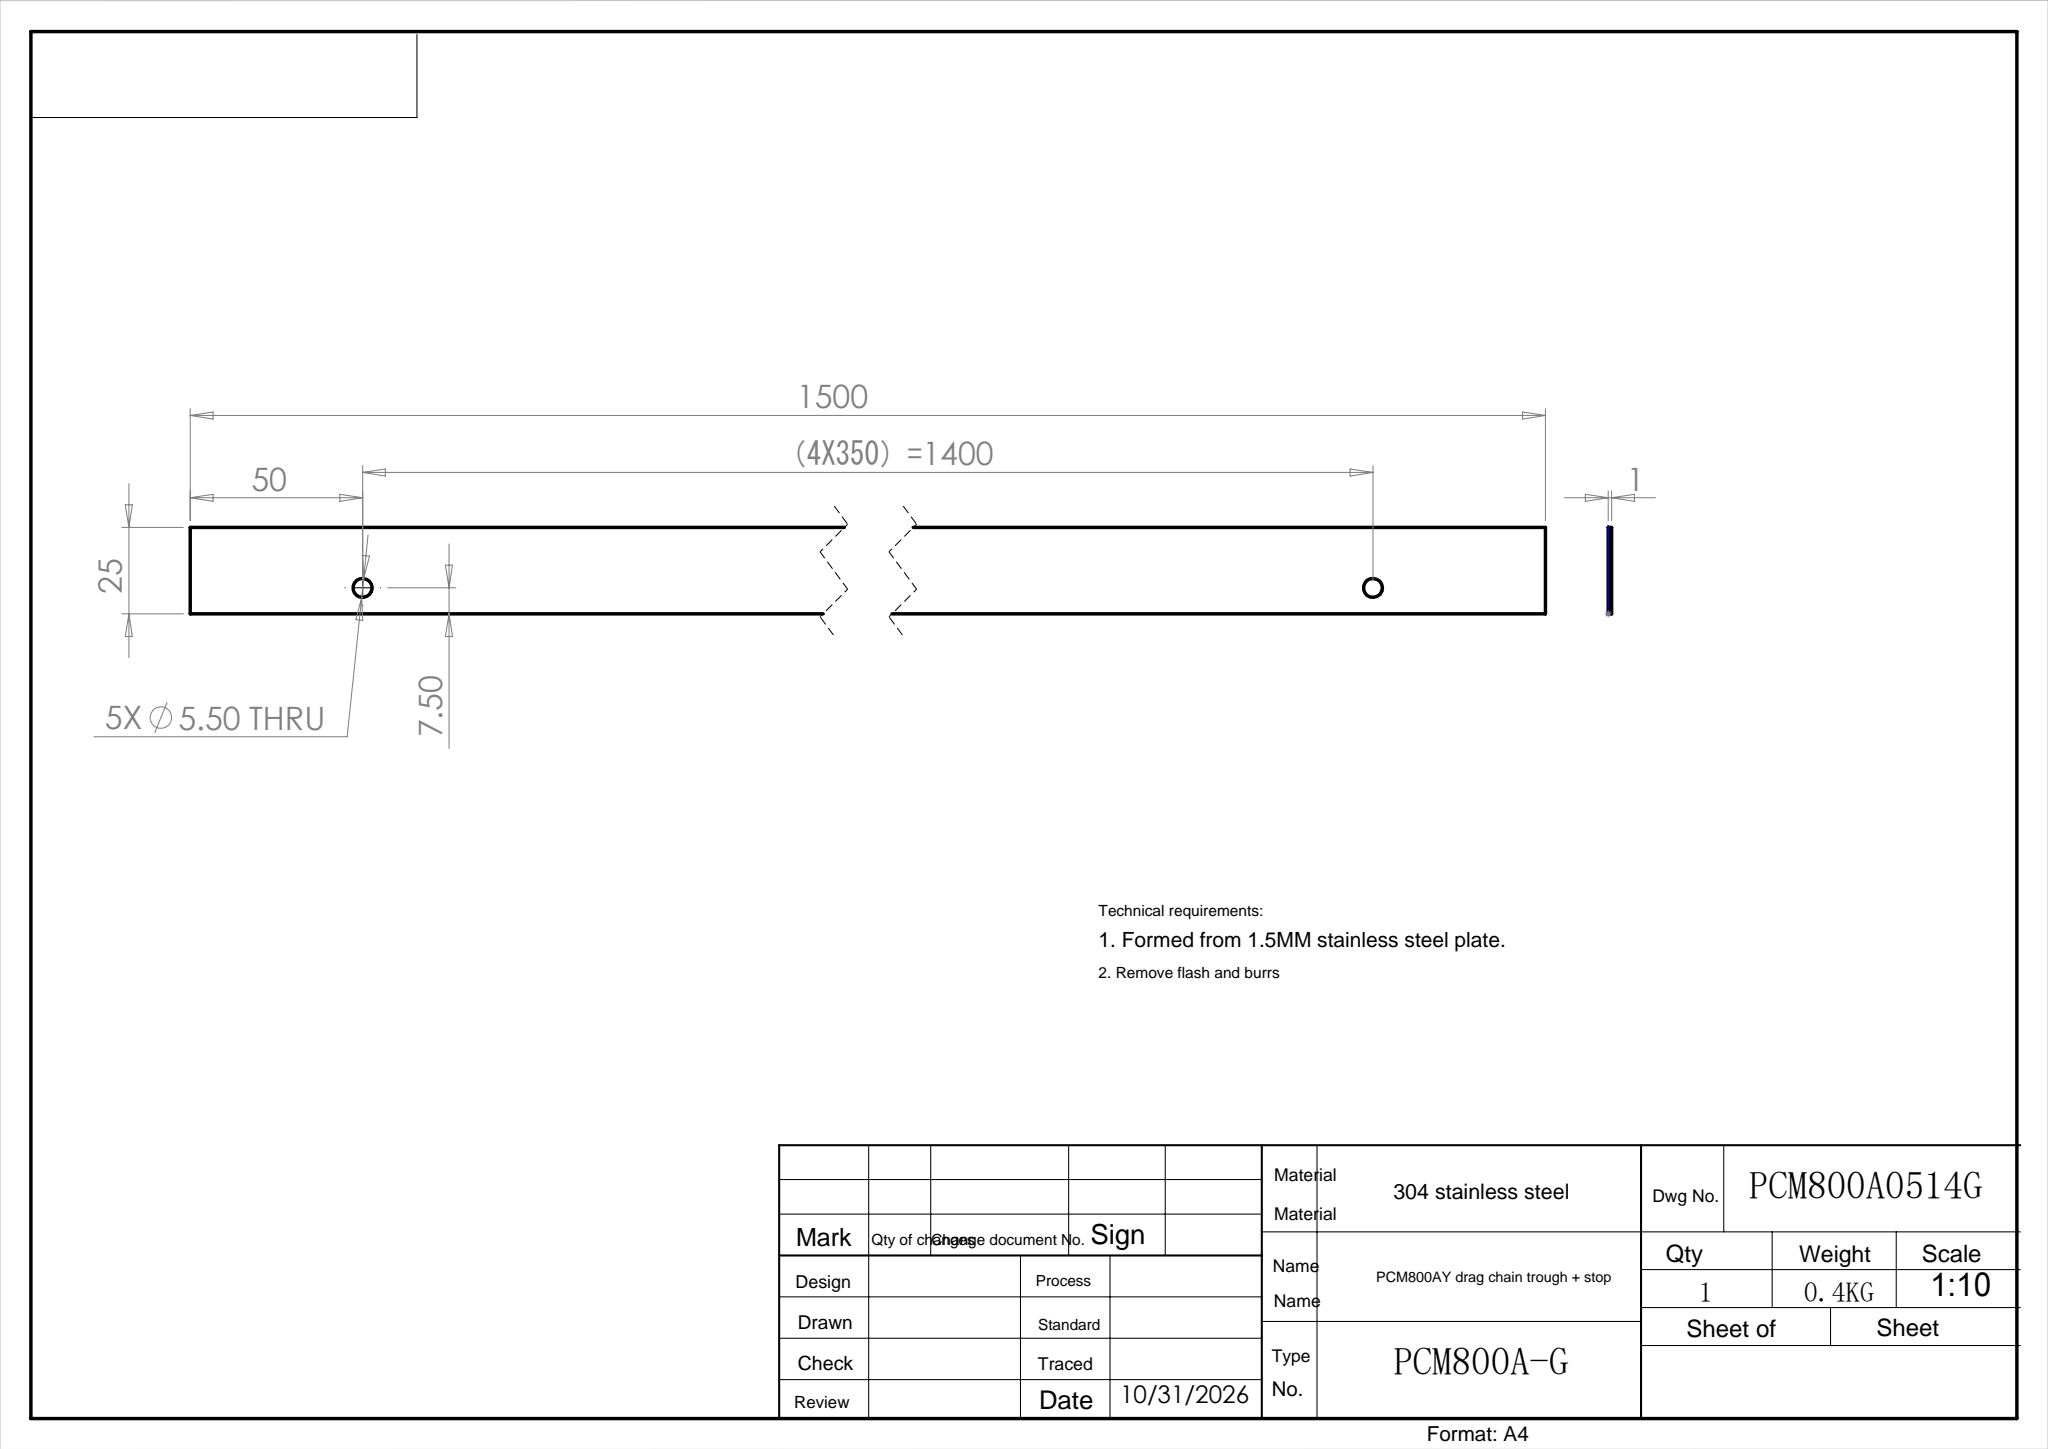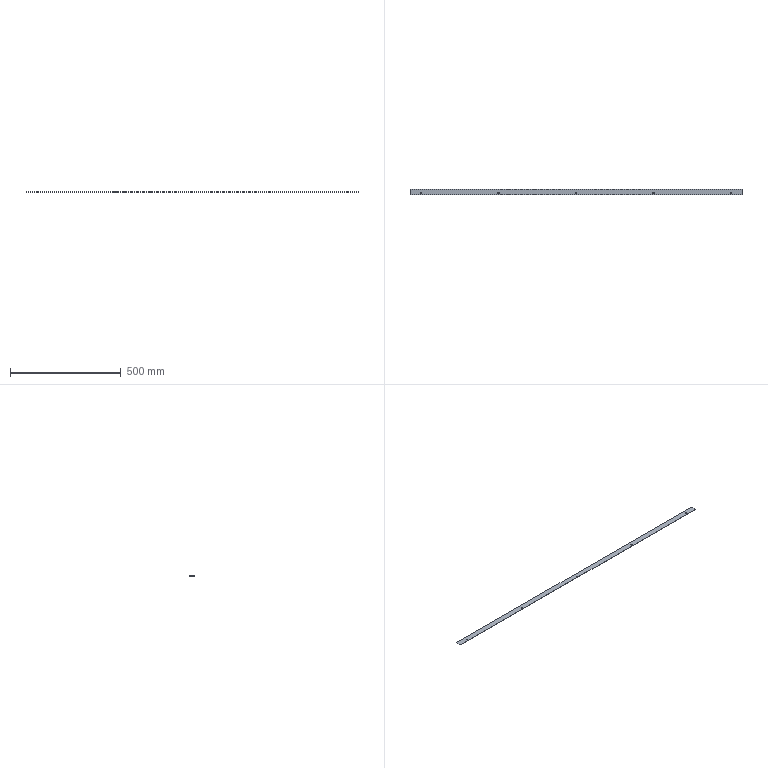Part | SolidWorks | features Extrusion 1, ICE 1 | 1 solid | 16 faces | box 1500 x 25 x 1 mm | volume 37381 mm3 | cylinder 10 | plane 6 | commonest cylinder face diameters 5.5 x10
STEP:
#1=CARTESIAN_POINT('',(1452.75,7.5,0.));
#2=VERTEX_POINT('',#1);
#3=CARTESIAN_POINT('',(1447.25,7.5,0.));
#4=VERTEX_POINT('',#3);
#5=CARTESIAN_POINT('',(1450.,7.5,0.));
#6=DIRECTION('',(0.,0.,-1.));
#7=DIRECTION('',(-1.,0.,0.));
#8=AXIS2_PLACEMENT_3D('',#5,#6,#7);
#9=CIRCLE('',#8,2.75);
#10=EDGE_CURVE('',#2,#4,#9,.T.);
#11=ORIENTED_EDGE('',*,*,#10,.T.);
#12=CARTESIAN_POINT('',(1447.25,7.5,1.));
#13=VERTEX_POINT('',#12);
#14=CARTESIAN_POINT('',(1447.25,7.5,-9.));
#15=DIRECTION('',(0.,0.,1.));
#16=VECTOR('',#15,1000.);
#17=LINE('',#14,#16);
#18=EDGE_CURVE('',#4,#13,#17,.T.);
#19=ORIENTED_EDGE('',*,*,#18,.T.);
#20=CARTESIAN_POINT('',(1452.75,7.5,1.));
#21=VERTEX_POINT('',#20);
#22=CARTESIAN_POINT('',(1450.,7.5,1.));
#23=DIRECTION('',(0.,0.,1.));
#24=DIRECTION('',(1.,0.,0.));
#25=AXIS2_PLACEMENT_3D('',#22,#23,#24);
#26=CIRCLE('',#25,2.75);
#27=EDGE_CURVE('',#13,#21,#26,.T.);
#28=ORIENTED_EDGE('',*,*,#27,.T.);
#29=CARTESIAN_POINT('',(1452.75,7.5,-9.));
#30=DIRECTION('',(0.,0.,1.));
#31=VECTOR('',#30,1000.);
#32=LINE('',#29,#31);
#33=EDGE_CURVE('',#2,#21,#32,.T.);
#34=ORIENTED_EDGE('',*,*,#33,.F.);
#35=EDGE_LOOP('',(#11,#19,#28,#34));
#36=FACE_OUTER_BOUND('',#35,.T.);
#37=CARTESIAN_POINT('',(1450.,7.5,-9.));
#38=DIRECTION('',(0.,0.,1.));
#39=DIRECTION('',(1.,0.,0.));
#40=AXIS2_PLACEMENT_3D('',#37,#38,#39);
#41=CYLINDRICAL_SURFACE('',#40,2.75);
#42=ADVANCED_FACE('',(#36),#41,.F.);
#43=CARTESIAN_POINT('',(1102.75,7.5,0.));
#44=VERTEX_POINT('',#43);
#45=CARTESIAN_POINT('',(1097.25,7.5,0.));
#46=VERTEX_POINT('',#45);
#47=CARTESIAN_POINT('',(1100.,7.5,0.));
#48=DIRECTION('',(0.,0.,-1.));
#49=DIRECTION('',(-1.,0.,0.));
#50=AXIS2_PLACEMENT_3D('',#47,#48,#49);
#51=CIRCLE('',#50,2.75);
#52=EDGE_CURVE('',#44,#46,#51,.T.);
#53=ORIENTED_EDGE('',*,*,#52,.T.);
#54=CARTESIAN_POINT('',(1097.25,7.5,1.));
#55=VERTEX_POINT('',#54);
#56=CARTESIAN_POINT('',(1097.25,7.5,-9.));
#57=DIRECTION('',(0.,0.,1.));
#58=VECTOR('',#57,1000.);
#59=LINE('',#56,#58);
#60=EDGE_CURVE('',#46,#55,#59,.T.);
#61=ORIENTED_EDGE('',*,*,#60,.T.);
#62=CARTESIAN_POINT('',(1102.75,7.5,1.));
#63=VERTEX_POINT('',#62);
#64=CARTESIAN_POINT('',(1100.,7.5,1.));
#65=DIRECTION('',(0.,0.,1.));
#66=DIRECTION('',(1.,0.,0.));
#67=AXIS2_PLACEMENT_3D('',#64,#65,#66);
#68=CIRCLE('',#67,2.75);
#69=EDGE_CURVE('',#55,#63,#68,.T.);
#70=ORIENTED_EDGE('',*,*,#69,.T.);
#71=CARTESIAN_POINT('',(1102.75,7.5,-9.));
#72=DIRECTION('',(0.,0.,1.));
#73=VECTOR('',#72,1000.);
#74=LINE('',#71,#73);
#75=EDGE_CURVE('',#44,#63,#74,.T.);
#76=ORIENTED_EDGE('',*,*,#75,.F.);
#77=EDGE_LOOP('',(#53,#61,#70,#76));
#78=FACE_OUTER_BOUND('',#77,.T.);
#79=CARTESIAN_POINT('',(1100.,7.5,-9.));
#80=DIRECTION('',(0.,0.,1.));
#81=DIRECTION('',(1.,0.,0.));
#82=AXIS2_PLACEMENT_3D('',#79,#80,#81);
#83=CYLINDRICAL_SURFACE('',#82,2.75);
#84=ADVANCED_FACE('',(#78),#83,.F.);
#85=CARTESIAN_POINT('',(752.75,7.5,0.));
#86=VERTEX_POINT('',#85);
#87=CARTESIAN_POINT('',(747.25,7.5,0.));
#88=VERTEX_POINT('',#87);
#89=CARTESIAN_POINT('',(750.,7.5,0.));
#90=DIRECTION('',(0.,0.,-1.));
#91=DIRECTION('',(-1.,0.,0.));
#92=AXIS2_PLACEMENT_3D('',#89,#90,#91);
#93=CIRCLE('',#92,2.75);
#94=EDGE_CURVE('',#86,#88,#93,.T.);
#95=ORIENTED_EDGE('',*,*,#94,.T.);
#96=CARTESIAN_POINT('',(747.25,7.5,1.));
#97=VERTEX_POINT('',#96);
#98=CARTESIAN_POINT('',(747.25,7.5,-9.));
#99=DIRECTION('',(0.,0.,1.));
#100=VECTOR('',#99,1000.);
#101=LINE('',#98,#100);
#102=EDGE_CURVE('',#88,#97,#101,.T.);
#103=ORIENTED_EDGE('',*,*,#102,.T.);
#104=CARTESIAN_POINT('',(752.75,7.5,1.));
#105=VERTEX_POINT('',#104);
#106=CARTESIAN_POINT('',(750.,7.5,1.));
#107=DIRECTION('',(0.,0.,1.));
#108=DIRECTION('',(1.,0.,0.));
#109=AXIS2_PLACEMENT_3D('',#106,#107,#108);
#110=CIRCLE('',#109,2.75);
#111=EDGE_CURVE('',#97,#105,#110,.T.);
#112=ORIENTED_EDGE('',*,*,#111,.T.);
#113=CARTESIAN_POINT('',(752.75,7.5,-9.));
#114=DIRECTION('',(0.,0.,1.));
#115=VECTOR('',#114,1000.);
#116=LINE('',#113,#115);
#117=EDGE_CURVE('',#86,#105,#116,.T.);
#118=ORIENTED_EDGE('',*,*,#117,.F.);
#119=EDGE_LOOP('',(#95,#103,#112,#118));
#120=FACE_OUTER_BOUND('',#119,.T.);
#121=CARTESIAN_POINT('',(750.,7.5,-9.));
#122=DIRECTION('',(0.,0.,1.));
#123=DIRECTION('',(1.,0.,0.));
#124=AXIS2_PLACEMENT_3D('',#121,#122,#123);
#125=CYLINDRICAL_SURFACE('',#124,2.75);
#126=ADVANCED_FACE('',(#120),#125,.F.);
#127=CARTESIAN_POINT('',(402.75,7.5,0.));
#128=VERTEX_POINT('',#127);
#129=CARTESIAN_POINT('',(397.25,7.5,0.));
#130=VERTEX_POINT('',#129);
#131=CARTESIAN_POINT('',(400.,7.5,0.));
#132=DIRECTION('',(0.,0.,-1.));
#133=DIRECTION('',(-1.,0.,0.));
#134=AXIS2_PLACEMENT_3D('',#131,#132,#133);
#135=CIRCLE('',#134,2.75);
#136=EDGE_CURVE('',#128,#130,#135,.T.);
#137=ORIENTED_EDGE('',*,*,#136,.T.);
#138=CARTESIAN_POINT('',(397.25,7.5,1.));
#139=VERTEX_POINT('',#138);
#140=CARTESIAN_POINT('',(397.25,7.5,-9.));
#141=DIRECTION('',(0.,0.,1.));
#142=VECTOR('',#141,1000.);
#143=LINE('',#140,#142);
#144=EDGE_CURVE('',#130,#139,#143,.T.);
#145=ORIENTED_EDGE('',*,*,#144,.T.);
#146=CARTESIAN_POINT('',(402.75,7.5,1.));
#147=VERTEX_POINT('',#146);
#148=CARTESIAN_POINT('',(400.,7.5,1.));
#149=DIRECTION('',(0.,0.,1.));
#150=DIRECTION('',(1.,0.,0.));
#151=AXIS2_PLACEMENT_3D('',#148,#149,#150);
#152=CIRCLE('',#151,2.75);
#153=EDGE_CURVE('',#139,#147,#152,.T.);
#154=ORIENTED_EDGE('',*,*,#153,.T.);
#155=CARTESIAN_POINT('',(402.75,7.5,-9.));
#156=DIRECTION('',(0.,0.,1.));
#157=VECTOR('',#156,1000.);
#158=LINE('',#155,#157);
#159=EDGE_CURVE('',#128,#147,#158,.T.);
#160=ORIENTED_EDGE('',*,*,#159,.F.);
#161=EDGE_LOOP('',(#137,#145,#154,#160));
#162=FACE_OUTER_BOUND('',#161,.T.);
#163=CARTESIAN_POINT('',(400.,7.5,-9.));
#164=DIRECTION('',(0.,0.,1.));
#165=DIRECTION('',(1.,0.,0.));
#166=AXIS2_PLACEMENT_3D('',#163,#164,#165);
#167=CYLINDRICAL_SURFACE('',#166,2.75);
#168=ADVANCED_FACE('',(#162),#167,.F.);
#169=CARTESIAN_POINT('',(52.75,7.5,0.));
#170=VERTEX_POINT('',#169);
#171=CARTESIAN_POINT('',(47.25,7.5,0.));
#172=VERTEX_POINT('',#171);
#173=CARTESIAN_POINT('',(50.,7.5,0.));
#174=DIRECTION('',(0.,0.,-1.));
#175=DIRECTION('',(-1.,0.,0.));
#176=AXIS2_PLACEMENT_3D('',#173,#174,#175);
#177=CIRCLE('',#176,2.75);
#178=EDGE_CURVE('',#170,#172,#177,.T.);
#179=ORIENTED_EDGE('',*,*,#178,.T.);
#180=CARTESIAN_POINT('',(47.25,7.5,1.));
#181=VERTEX_POINT('',#180);
#182=CARTESIAN_POINT('',(47.25,7.5,-9.));
#183=DIRECTION('',(0.,0.,1.));
#184=VECTOR('',#183,1000.);
#185=LINE('',#182,#184);
#186=EDGE_CURVE('',#172,#181,#185,.T.);
#187=ORIENTED_EDGE('',*,*,#186,.T.);
#188=CARTESIAN_POINT('',(52.75,7.5,1.));
#189=VERTEX_POINT('',#188);
#190=CARTESIAN_POINT('',(50.,7.5,1.));
#191=DIRECTION('',(0.,0.,1.));
#192=DIRECTION('',(1.,0.,0.));
#193=AXIS2_PLACEMENT_3D('',#190,#191,#192);
#194=CIRCLE('',#193,2.75);
#195=EDGE_CURVE('',#181,#189,#194,.T.);
#196=ORIENTED_EDGE('',*,*,#195,.T.);
#197=CARTESIAN_POINT('',(52.75,7.5,-9.));
#198=DIRECTION('',(0.,0.,1.));
#199=VECTOR('',#198,1000.);
#200=LINE('',#197,#199);
#201=EDGE_CURVE('',#170,#189,#200,.T.);
#202=ORIENTED_EDGE('',*,*,#201,.F.);
#203=EDGE_LOOP('',(#179,#187,#196,#202));
#204=FACE_OUTER_BOUND('',#203,.T.);
#205=CARTESIAN_POINT('',(50.,7.5,-9.));
#206=DIRECTION('',(0.,0.,1.));
#207=DIRECTION('',(1.,0.,0.));
#208=AXIS2_PLACEMENT_3D('',#205,#206,#207);
#209=CYLINDRICAL_SURFACE('',#208,2.75);
#210=ADVANCED_FACE('',(#204),#209,.F.);
#211=CARTESIAN_POINT('',(0.,25.,0.));
#212=VERTEX_POINT('',#211);
#213=CARTESIAN_POINT('',(0.,0.,0.));
#214=VERTEX_POINT('',#213);
#215=CARTESIAN_POINT('',(0.,0.,0.));
#216=DIRECTION('',(0.,-1.,0.));
#217=VECTOR('',#216,1000.);
#218=LINE('',#215,#217);
#219=EDGE_CURVE('',#212,#214,#218,.T.);
#220=ORIENTED_EDGE('',*,*,#219,.T.);
#221=CARTESIAN_POINT('',(0.,0.,1.));
#222=VERTEX_POINT('',#221);
#223=CARTESIAN_POINT('',(0.,0.,1.));
#224=DIRECTION('',(0.,0.,-1.));
#225=VECTOR('',#224,1000.);
#226=LINE('',#223,#225);
#227=EDGE_CURVE('',#222,#214,#226,.T.);
#228=ORIENTED_EDGE('',*,*,#227,.F.);
#229=CARTESIAN_POINT('',(0.,25.,1.));
#230=VERTEX_POINT('',#229);
#231=CARTESIAN_POINT('',(0.,0.,1.));
#232=DIRECTION('',(0.,-1.,0.));
#233=VECTOR('',#232,1000.);
#234=LINE('',#231,#233);
#235=EDGE_CURVE('',#230,#222,#234,.T.);
#236=ORIENTED_EDGE('',*,*,#235,.F.);
#237=CARTESIAN_POINT('',(0.,25.,1.));
#238=DIRECTION('',(0.,0.,-1.));
#239=VECTOR('',#238,1000.);
#240=LINE('',#237,#239);
#241=EDGE_CURVE('',#230,#212,#240,.T.);
#242=ORIENTED_EDGE('',*,*,#241,.T.);
#243=EDGE_LOOP('',(#220,#228,#236,#242));
#244=FACE_OUTER_BOUND('',#243,.T.);
#245=CARTESIAN_POINT('',(0.,0.,1.));
#246=DIRECTION('',(1.,0.,0.));
#247=DIRECTION('',(0.,0.,-1.));
#248=AXIS2_PLACEMENT_3D('',#245,#246,#247);
#249=PLANE('',#248);
#250=ADVANCED_FACE('',(#244),#249,.F.);
#251=CARTESIAN_POINT('',(1500.,0.,0.));
#252=VERTEX_POINT('',#251);
#253=CARTESIAN_POINT('',(0.,0.,0.));
#254=DIRECTION('',(1.,0.,0.));
#255=VECTOR('',#254,1000.);
#256=LINE('',#253,#255);
#257=EDGE_CURVE('',#214,#252,#256,.T.);
#258=ORIENTED_EDGE('',*,*,#257,.T.);
#259=CARTESIAN_POINT('',(1500.,0.,1.));
#260=VERTEX_POINT('',#259);
#261=CARTESIAN_POINT('',(1500.,0.,1.));
#262=DIRECTION('',(0.,0.,-1.));
#263=VECTOR('',#262,1000.);
#264=LINE('',#261,#263);
#265=EDGE_CURVE('',#260,#252,#264,.T.);
#266=ORIENTED_EDGE('',*,*,#265,.F.);
#267=CARTESIAN_POINT('',(0.,0.,1.));
#268=DIRECTION('',(1.,0.,0.));
#269=VECTOR('',#268,1000.);
#270=LINE('',#267,#269);
#271=EDGE_CURVE('',#222,#260,#270,.T.);
#272=ORIENTED_EDGE('',*,*,#271,.F.);
#273=ORIENTED_EDGE('',*,*,#227,.T.);
#274=EDGE_LOOP('',(#258,#266,#272,#273));
#275=FACE_OUTER_BOUND('',#274,.T.);
#276=CARTESIAN_POINT('',(0.,0.,1.));
#277=DIRECTION('',(0.,1.,0.));
#278=DIRECTION('',(0.,0.,1.));
#279=AXIS2_PLACEMENT_3D('',#276,#277,#278);
#280=PLANE('',#279);
#281=ADVANCED_FACE('',(#275),#280,.F.);
#282=CARTESIAN_POINT('',(1500.,25.,0.));
#283=VERTEX_POINT('',#282);
#284=CARTESIAN_POINT('',(1500.,0.,0.));
#285=DIRECTION('',(0.,1.,0.));
#286=VECTOR('',#285,1000.);
#287=LINE('',#284,#286);
#288=EDGE_CURVE('',#252,#283,#287,.T.);
#289=ORIENTED_EDGE('',*,*,#288,.T.);
#290=CARTESIAN_POINT('',(1500.,25.,1.));
#291=VERTEX_POINT('',#290);
#292=CARTESIAN_POINT('',(1500.,25.,1.));
#293=DIRECTION('',(0.,0.,-1.));
#294=VECTOR('',#293,1000.);
#295=LINE('',#292,#294);
#296=EDGE_CURVE('',#291,#283,#295,.T.);
#297=ORIENTED_EDGE('',*,*,#296,.F.);
#298=CARTESIAN_POINT('',(1500.,0.,1.));
#299=DIRECTION('',(0.,1.,0.));
#300=VECTOR('',#299,1000.);
#301=LINE('',#298,#300);
#302=EDGE_CURVE('',#260,#291,#301,.T.);
#303=ORIENTED_EDGE('',*,*,#302,.F.);
#304=ORIENTED_EDGE('',*,*,#265,.T.);
#305=EDGE_LOOP('',(#289,#297,#303,#304));
#306=FACE_OUTER_BOUND('',#305,.T.);
#307=CARTESIAN_POINT('',(1500.,0.,1.));
#308=DIRECTION('',(-1.,0.,0.));
#309=DIRECTION('',(0.,0.,1.));
#310=AXIS2_PLACEMENT_3D('',#307,#308,#309);
#311=PLANE('',#310);
#312=ADVANCED_FACE('',(#306),#311,.F.);
#313=CARTESIAN_POINT('',(0.,25.,0.));
#314=DIRECTION('',(-1.,0.,0.));
#315=VECTOR('',#314,1000.);
#316=LINE('',#313,#315);
#317=EDGE_CURVE('',#283,#212,#316,.T.);
#318=ORIENTED_EDGE('',*,*,#317,.T.);
#319=ORIENTED_EDGE('',*,*,#241,.F.);
#320=CARTESIAN_POINT('',(0.,25.,1.));
#321=DIRECTION('',(-1.,0.,0.));
#322=VECTOR('',#321,1000.);
#323=LINE('',#320,#322);
#324=EDGE_CURVE('',#291,#230,#323,.T.);
#325=ORIENTED_EDGE('',*,*,#324,.F.);
#326=ORIENTED_EDGE('',*,*,#296,.T.);
#327=EDGE_LOOP('',(#318,#319,#325,#326));
#328=FACE_OUTER_BOUND('',#327,.T.);
#329=CARTESIAN_POINT('',(0.,25.,1.));
#330=DIRECTION('',(0.,-1.,0.));
#331=DIRECTION('',(0.,0.,-1.));
#332=AXIS2_PLACEMENT_3D('',#329,#330,#331);
#333=PLANE('',#332);
#334=ADVANCED_FACE('',(#328),#333,.F.);
#335=CARTESIAN_POINT('',(1450.,7.5,1.));
#336=DIRECTION('',(0.,0.,1.));
#337=DIRECTION('',(1.,0.,0.));
#338=AXIS2_PLACEMENT_3D('',#335,#336,#337);
#339=CIRCLE('',#338,2.75);
#340=EDGE_CURVE('',#21,#13,#339,.T.);
#341=ORIENTED_EDGE('',*,*,#340,.F.);
#342=ORIENTED_EDGE('',*,*,#27,.F.);
#343=EDGE_LOOP('',(#341,#342));
#344=FACE_BOUND('',#343,.T.);
#345=CARTESIAN_POINT('',(1100.,7.5,1.));
#346=DIRECTION('',(0.,0.,1.));
#347=DIRECTION('',(1.,0.,0.));
#348=AXIS2_PLACEMENT_3D('',#345,#346,#347);
#349=CIRCLE('',#348,2.75);
#350=EDGE_CURVE('',#63,#55,#349,.T.);
#351=ORIENTED_EDGE('',*,*,#350,.F.);
#352=ORIENTED_EDGE('',*,*,#69,.F.);
#353=EDGE_LOOP('',(#351,#352));
#354=FACE_BOUND('',#353,.T.);
#355=CARTESIAN_POINT('',(750.,7.5,1.));
#356=DIRECTION('',(0.,0.,1.));
#357=DIRECTION('',(1.,0.,0.));
#358=AXIS2_PLACEMENT_3D('',#355,#356,#357);
#359=CIRCLE('',#358,2.75);
#360=EDGE_CURVE('',#105,#97,#359,.T.);
#361=ORIENTED_EDGE('',*,*,#360,.F.);
#362=ORIENTED_EDGE('',*,*,#111,.F.);
#363=EDGE_LOOP('',(#361,#362));
#364=FACE_BOUND('',#363,.T.);
#365=CARTESIAN_POINT('',(400.,7.5,1.));
#366=DIRECTION('',(0.,0.,1.));
#367=DIRECTION('',(1.,0.,0.));
#368=AXIS2_PLACEMENT_3D('',#365,#366,#367);
#369=CIRCLE('',#368,2.75);
#370=EDGE_CURVE('',#147,#139,#369,.T.);
#371=ORIENTED_EDGE('',*,*,#370,.F.);
#372=ORIENTED_EDGE('',*,*,#153,.F.);
#373=EDGE_LOOP('',(#371,#372));
#374=FACE_BOUND('',#373,.T.);
#375=CARTESIAN_POINT('',(50.,7.5,1.));
#376=DIRECTION('',(0.,0.,1.));
#377=DIRECTION('',(1.,0.,0.));
#378=AXIS2_PLACEMENT_3D('',#375,#376,#377);
#379=CIRCLE('',#378,2.75);
#380=EDGE_CURVE('',#189,#181,#379,.T.);
#381=ORIENTED_EDGE('',*,*,#380,.F.);
#382=ORIENTED_EDGE('',*,*,#195,.F.);
#383=EDGE_LOOP('',(#381,#382));
#384=FACE_BOUND('',#383,.T.);
#385=ORIENTED_EDGE('',*,*,#235,.T.);
#386=ORIENTED_EDGE('',*,*,#271,.T.);
#387=ORIENTED_EDGE('',*,*,#302,.T.);
#388=ORIENTED_EDGE('',*,*,#324,.T.);
#389=EDGE_LOOP('',(#385,#386,#387,#388));
#390=FACE_OUTER_BOUND('',#389,.T.);
#391=CARTESIAN_POINT('',(0.,25.,1.));
#392=DIRECTION('',(0.,0.,-1.));
#393=DIRECTION('',(-1.,0.,0.));
#394=AXIS2_PLACEMENT_3D('',#391,#392,#393);
#395=PLANE('',#394);
#396=ADVANCED_FACE('',(#344,#354,#364,#374,#384,#390),#395,.F.);
#397=ORIENTED_EDGE('',*,*,#10,.F.);
#398=CARTESIAN_POINT('',(1450.,7.5,0.));
#399=DIRECTION('',(0.,0.,-1.));
#400=DIRECTION('',(-1.,0.,0.));
#401=AXIS2_PLACEMENT_3D('',#398,#399,#400);
#402=CIRCLE('',#401,2.75);
#403=EDGE_CURVE('',#4,#2,#402,.T.);
#404=ORIENTED_EDGE('',*,*,#403,.F.);
#405=EDGE_LOOP('',(#397,#404));
#406=FACE_BOUND('',#405,.T.);
#407=ORIENTED_EDGE('',*,*,#52,.F.);
#408=CARTESIAN_POINT('',(1100.,7.5,0.));
#409=DIRECTION('',(0.,0.,-1.));
#410=DIRECTION('',(-1.,0.,0.));
#411=AXIS2_PLACEMENT_3D('',#408,#409,#410);
#412=CIRCLE('',#411,2.75);
#413=EDGE_CURVE('',#46,#44,#412,.T.);
#414=ORIENTED_EDGE('',*,*,#413,.F.);
#415=EDGE_LOOP('',(#407,#414));
#416=FACE_BOUND('',#415,.T.);
#417=ORIENTED_EDGE('',*,*,#94,.F.);
#418=CARTESIAN_POINT('',(750.,7.5,0.));
#419=DIRECTION('',(0.,0.,-1.));
#420=DIRECTION('',(-1.,0.,0.));
#421=AXIS2_PLACEMENT_3D('',#418,#419,#420);
#422=CIRCLE('',#421,2.75);
#423=EDGE_CURVE('',#88,#86,#422,.T.);
#424=ORIENTED_EDGE('',*,*,#423,.F.);
#425=EDGE_LOOP('',(#417,#424));
#426=FACE_BOUND('',#425,.T.);
#427=ORIENTED_EDGE('',*,*,#136,.F.);
#428=CARTESIAN_POINT('',(400.,7.5,0.));
#429=DIRECTION('',(0.,0.,-1.));
#430=DIRECTION('',(-1.,0.,0.));
#431=AXIS2_PLACEMENT_3D('',#428,#429,#430);
#432=CIRCLE('',#431,2.75);
#433=EDGE_CURVE('',#130,#128,#432,.T.);
#434=ORIENTED_EDGE('',*,*,#433,.F.);
#435=EDGE_LOOP('',(#427,#434));
#436=FACE_BOUND('',#435,.T.);
#437=ORIENTED_EDGE('',*,*,#178,.F.);
#438=CARTESIAN_POINT('',(50.,7.5,0.));
#439=DIRECTION('',(0.,0.,-1.));
#440=DIRECTION('',(-1.,0.,0.));
#441=AXIS2_PLACEMENT_3D('',#438,#439,#440);
#442=CIRCLE('',#441,2.75);
#443=EDGE_CURVE('',#172,#170,#442,.T.);
#444=ORIENTED_EDGE('',*,*,#443,.F.);
#445=EDGE_LOOP('',(#437,#444));
#446=FACE_BOUND('',#445,.T.);
#447=ORIENTED_EDGE('',*,*,#219,.F.);
#448=ORIENTED_EDGE('',*,*,#317,.F.);
#449=ORIENTED_EDGE('',*,*,#288,.F.);
#450=ORIENTED_EDGE('',*,*,#257,.F.);
#451=EDGE_LOOP('',(#447,#448,#449,#450));
#452=FACE_OUTER_BOUND('',#451,.T.);
#453=CARTESIAN_POINT('',(0.,25.,0.));
#454=DIRECTION('',(0.,0.,-1.));
#455=DIRECTION('',(-1.,0.,0.));
#456=AXIS2_PLACEMENT_3D('',#453,#454,#455);
#457=PLANE('',#456);
#458=ADVANCED_FACE('',(#406,#416,#426,#436,#446,#452),#457,.T.);
#459=ORIENTED_EDGE('',*,*,#186,.F.);
#460=ORIENTED_EDGE('',*,*,#443,.T.);
#461=ORIENTED_EDGE('',*,*,#201,.T.);
#462=ORIENTED_EDGE('',*,*,#380,.T.);
#463=EDGE_LOOP('',(#459,#460,#461,#462));
#464=FACE_OUTER_BOUND('',#463,.T.);
#465=CARTESIAN_POINT('',(50.,7.5,-9.));
#466=DIRECTION('',(0.,0.,1.));
#467=DIRECTION('',(1.,0.,0.));
#468=AXIS2_PLACEMENT_3D('',#465,#466,#467);
#469=CYLINDRICAL_SURFACE('',#468,2.75);
#470=ADVANCED_FACE('',(#464),#469,.F.);
#471=ORIENTED_EDGE('',*,*,#144,.F.);
#472=ORIENTED_EDGE('',*,*,#433,.T.);
#473=ORIENTED_EDGE('',*,*,#159,.T.);
#474=ORIENTED_EDGE('',*,*,#370,.T.);
#475=EDGE_LOOP('',(#471,#472,#473,#474));
#476=FACE_OUTER_BOUND('',#475,.T.);
#477=CARTESIAN_POINT('',(400.,7.5,-9.));
#478=DIRECTION('',(0.,0.,1.));
#479=DIRECTION('',(1.,0.,0.));
#480=AXIS2_PLACEMENT_3D('',#477,#478,#479);
#481=CYLINDRICAL_SURFACE('',#480,2.75);
#482=ADVANCED_FACE('',(#476),#481,.F.);
#483=ORIENTED_EDGE('',*,*,#102,.F.);
#484=ORIENTED_EDGE('',*,*,#423,.T.);
#485=ORIENTED_EDGE('',*,*,#117,.T.);
#486=ORIENTED_EDGE('',*,*,#360,.T.);
#487=EDGE_LOOP('',(#483,#484,#485,#486));
#488=FACE_OUTER_BOUND('',#487,.T.);
#489=CARTESIAN_POINT('',(750.,7.5,-9.));
#490=DIRECTION('',(0.,0.,1.));
#491=DIRECTION('',(1.,0.,0.));
#492=AXIS2_PLACEMENT_3D('',#489,#490,#491);
#493=CYLINDRICAL_SURFACE('',#492,2.75);
#494=ADVANCED_FACE('',(#488),#493,.F.);
#495=ORIENTED_EDGE('',*,*,#60,.F.);
#496=ORIENTED_EDGE('',*,*,#413,.T.);
#497=ORIENTED_EDGE('',*,*,#75,.T.);
#498=ORIENTED_EDGE('',*,*,#350,.T.);
#499=EDGE_LOOP('',(#495,#496,#497,#498));
#500=FACE_OUTER_BOUND('',#499,.T.);
#501=CARTESIAN_POINT('',(1100.,7.5,-9.));
#502=DIRECTION('',(0.,0.,1.));
#503=DIRECTION('',(1.,0.,0.));
#504=AXIS2_PLACEMENT_3D('',#501,#502,#503);
#505=CYLINDRICAL_SURFACE('',#504,2.75);
#506=ADVANCED_FACE('',(#500),#505,.F.);
#507=ORIENTED_EDGE('',*,*,#18,.F.);
#508=ORIENTED_EDGE('',*,*,#403,.T.);
#509=ORIENTED_EDGE('',*,*,#33,.T.);
#510=ORIENTED_EDGE('',*,*,#340,.T.);
#511=EDGE_LOOP('',(#507,#508,#509,#510));
#512=FACE_OUTER_BOUND('',#511,.T.);
#513=CARTESIAN_POINT('',(1450.,7.5,-9.));
#514=DIRECTION('',(0.,0.,1.));
#515=DIRECTION('',(1.,0.,0.));
#516=AXIS2_PLACEMENT_3D('',#513,#514,#515);
#517=CYLINDRICAL_SURFACE('',#516,2.75);
#518=ADVANCED_FACE('',(#512),#517,.F.);
#519=CLOSED_SHELL('',(#42,#84,#126,#168,#210,#250,#281,#312,#334,#396,#458,#470,#482,#494,#506,#518));
#520=MANIFOLD_SOLID_BREP('',#519);
#521=CARTESIAN_POINT('',(0.,0.,0.));
#522=DIRECTION('',(0.,0.,1.));
#523=DIRECTION('',(1.,0.,0.));
#524=AXIS2_PLACEMENT_3D('',#521,#522,#523);
#525=(LENGTH_UNIT()NAMED_UNIT(*)SI_UNIT(.MILLI.,.METRE.));
#526=UNCERTAINTY_MEASURE_WITH_UNIT(LENGTH_MEASURE(0.00001),#525,'','');
#527=(NAMED_UNIT(*)PLANE_ANGLE_UNIT()SI_UNIT($,.RADIAN.));
#528=(NAMED_UNIT(*)SI_UNIT($,.STERADIAN.)SOLID_ANGLE_UNIT());
#529=(GEOMETRIC_REPRESENTATION_CONTEXT(3)GLOBAL_UNCERTAINTY_ASSIGNED_CONTEXT((#526))GLOBAL_UNIT_ASSIGNED_CONTEXT((#525,#527,#528))REPRESENTATION_CONTEXT('',''));
#530=ADVANCED_BREP_SHAPE_REPRESENTATION('',(#520,#524),#529);